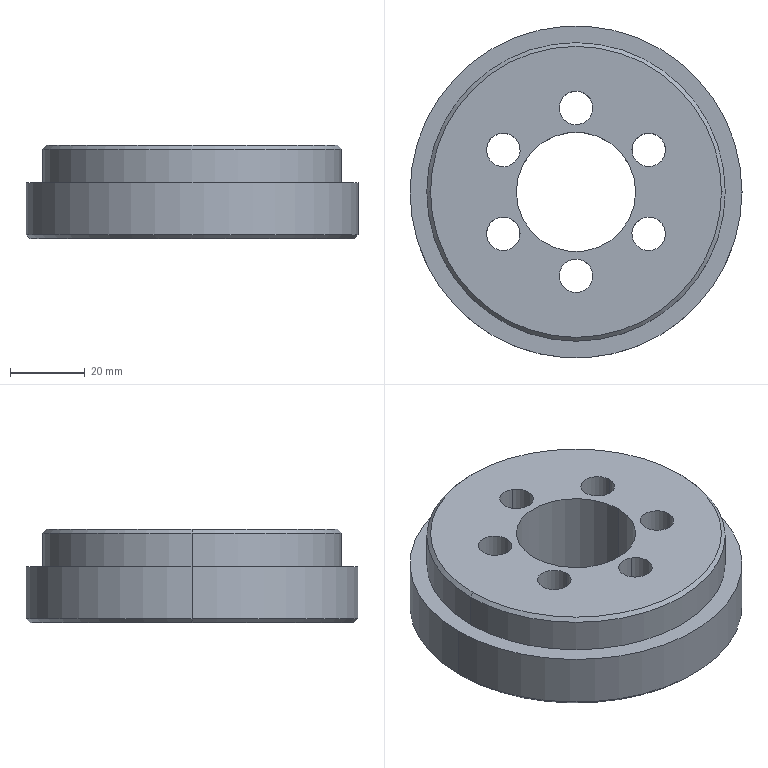Part | SolidWorks | features BaseBody 1 | 1 solid | 25 faces | box 89 x 89 x 25 mm | volume 113670 mm3 | cylinder 18 | cone 4 | plane 3 | commonest cylinder face diameters 9 x12 32 x2 80 x2 89 x2
STEP:
#1=CARTESIAN_POINT('',(-2.25,18.603,25.));
#2=VERTEX_POINT('',#1);
#3=CARTESIAN_POINT('',(2.25,26.397,25.));
#4=VERTEX_POINT('',#3);
#5=CARTESIAN_POINT('',(0.,22.5,25.));
#6=DIRECTION('',(0.,0.,1.));
#7=DIRECTION('',(0.5,0.866,0.));
#8=AXIS2_PLACEMENT_3D('',#5,#6,#7);
#9=CIRCLE('',#8,4.5);
#10=EDGE_CURVE('',#2,#4,#9,.T.);
#11=ORIENTED_EDGE('',*,*,#10,.T.);
#12=CARTESIAN_POINT('',(2.25,26.397,0.));
#13=VERTEX_POINT('',#12);
#14=CARTESIAN_POINT('',(2.25,26.397,0.));
#15=DIRECTION('',(0.,0.,-1.));
#16=VECTOR('',#15,1000.);
#17=LINE('',#14,#16);
#18=EDGE_CURVE('',#4,#13,#17,.T.);
#19=ORIENTED_EDGE('',*,*,#18,.T.);
#20=CARTESIAN_POINT('',(-2.25,18.603,0.));
#21=VERTEX_POINT('',#20);
#22=CARTESIAN_POINT('',(0.,22.5,0.));
#23=DIRECTION('',(0.,0.,-1.));
#24=DIRECTION('',(-0.5,-0.866,0.));
#25=AXIS2_PLACEMENT_3D('',#22,#23,#24);
#26=CIRCLE('',#25,4.5);
#27=EDGE_CURVE('',#13,#21,#26,.T.);
#28=ORIENTED_EDGE('',*,*,#27,.T.);
#29=CARTESIAN_POINT('',(-2.25,18.603,0.));
#30=DIRECTION('',(0.,0.,-1.));
#31=VECTOR('',#30,1000.);
#32=LINE('',#29,#31);
#33=EDGE_CURVE('',#2,#21,#32,.T.);
#34=ORIENTED_EDGE('',*,*,#33,.F.);
#35=EDGE_LOOP('',(#11,#19,#28,#34));
#36=FACE_OUTER_BOUND('',#35,.T.);
#37=CARTESIAN_POINT('',(0.,22.5,0.));
#38=DIRECTION('',(0.,0.,-1.));
#39=DIRECTION('',(-0.5,-0.866,0.));
#40=AXIS2_PLACEMENT_3D('',#37,#38,#39);
#41=CYLINDRICAL_SURFACE('',#40,4.5);
#42=ADVANCED_FACE('',(#36),#41,.F.);
#43=CARTESIAN_POINT('',(-17.236,7.353,25.));
#44=VERTEX_POINT('',#43);
#45=CARTESIAN_POINT('',(-21.736,15.147,25.));
#46=VERTEX_POINT('',#45);
#47=CARTESIAN_POINT('',(-19.486,11.25,25.));
#48=DIRECTION('',(0.,0.,1.));
#49=DIRECTION('',(-0.5,0.866,0.));
#50=AXIS2_PLACEMENT_3D('',#47,#48,#49);
#51=CIRCLE('',#50,4.5);
#52=EDGE_CURVE('',#44,#46,#51,.T.);
#53=ORIENTED_EDGE('',*,*,#52,.T.);
#54=CARTESIAN_POINT('',(-21.736,15.147,0.));
#55=VERTEX_POINT('',#54);
#56=CARTESIAN_POINT('',(-21.736,15.147,0.));
#57=DIRECTION('',(0.,0.,-1.));
#58=VECTOR('',#57,1000.);
#59=LINE('',#56,#58);
#60=EDGE_CURVE('',#46,#55,#59,.T.);
#61=ORIENTED_EDGE('',*,*,#60,.T.);
#62=CARTESIAN_POINT('',(-17.236,7.353,0.));
#63=VERTEX_POINT('',#62);
#64=CARTESIAN_POINT('',(-19.486,11.25,0.));
#65=DIRECTION('',(0.,0.,-1.));
#66=DIRECTION('',(0.5,-0.866,0.));
#67=AXIS2_PLACEMENT_3D('',#64,#65,#66);
#68=CIRCLE('',#67,4.5);
#69=EDGE_CURVE('',#55,#63,#68,.T.);
#70=ORIENTED_EDGE('',*,*,#69,.T.);
#71=CARTESIAN_POINT('',(-17.236,7.353,0.));
#72=DIRECTION('',(0.,0.,-1.));
#73=VECTOR('',#72,1000.);
#74=LINE('',#71,#73);
#75=EDGE_CURVE('',#44,#63,#74,.T.);
#76=ORIENTED_EDGE('',*,*,#75,.F.);
#77=EDGE_LOOP('',(#53,#61,#70,#76));
#78=FACE_OUTER_BOUND('',#77,.T.);
#79=CARTESIAN_POINT('',(-19.486,11.25,0.));
#80=DIRECTION('',(0.,0.,-1.));
#81=DIRECTION('',(0.5,-0.866,0.));
#82=AXIS2_PLACEMENT_3D('',#79,#80,#81);
#83=CYLINDRICAL_SURFACE('',#82,4.5);
#84=ADVANCED_FACE('',(#78),#83,.F.);
#85=CARTESIAN_POINT('',(-14.986,-11.25,25.));
#86=VERTEX_POINT('',#85);
#87=CARTESIAN_POINT('',(-23.986,-11.25,25.));
#88=VERTEX_POINT('',#87);
#89=CARTESIAN_POINT('',(-19.486,-11.25,25.));
#90=DIRECTION('',(0.,0.,1.));
#91=DIRECTION('',(-1.,0.,0.));
#92=AXIS2_PLACEMENT_3D('',#89,#90,#91);
#93=CIRCLE('',#92,4.5);
#94=EDGE_CURVE('',#86,#88,#93,.T.);
#95=ORIENTED_EDGE('',*,*,#94,.T.);
#96=CARTESIAN_POINT('',(-23.986,-11.25,0.));
#97=VERTEX_POINT('',#96);
#98=CARTESIAN_POINT('',(-23.986,-11.25,0.));
#99=DIRECTION('',(0.,0.,-1.));
#100=VECTOR('',#99,1000.);
#101=LINE('',#98,#100);
#102=EDGE_CURVE('',#88,#97,#101,.T.);
#103=ORIENTED_EDGE('',*,*,#102,.T.);
#104=CARTESIAN_POINT('',(-14.986,-11.25,0.));
#105=VERTEX_POINT('',#104);
#106=CARTESIAN_POINT('',(-19.486,-11.25,0.));
#107=DIRECTION('',(0.,0.,-1.));
#108=DIRECTION('',(1.,0.,0.));
#109=AXIS2_PLACEMENT_3D('',#106,#107,#108);
#110=CIRCLE('',#109,4.5);
#111=EDGE_CURVE('',#97,#105,#110,.T.);
#112=ORIENTED_EDGE('',*,*,#111,.T.);
#113=CARTESIAN_POINT('',(-14.986,-11.25,0.));
#114=DIRECTION('',(0.,0.,-1.));
#115=VECTOR('',#114,1000.);
#116=LINE('',#113,#115);
#117=EDGE_CURVE('',#86,#105,#116,.T.);
#118=ORIENTED_EDGE('',*,*,#117,.F.);
#119=EDGE_LOOP('',(#95,#103,#112,#118));
#120=FACE_OUTER_BOUND('',#119,.T.);
#121=CARTESIAN_POINT('',(-19.486,-11.25,0.));
#122=DIRECTION('',(0.,0.,-1.));
#123=DIRECTION('',(1.,0.,0.));
#124=AXIS2_PLACEMENT_3D('',#121,#122,#123);
#125=CYLINDRICAL_SURFACE('',#124,4.5);
#126=ADVANCED_FACE('',(#120),#125,.F.);
#127=CARTESIAN_POINT('',(2.25,-18.603,25.));
#128=VERTEX_POINT('',#127);
#129=CARTESIAN_POINT('',(-2.25,-26.397,25.));
#130=VERTEX_POINT('',#129);
#131=CARTESIAN_POINT('',(0.,-22.5,25.));
#132=DIRECTION('',(0.,0.,1.));
#133=DIRECTION('',(-0.5,-0.866,0.));
#134=AXIS2_PLACEMENT_3D('',#131,#132,#133);
#135=CIRCLE('',#134,4.5);
#136=EDGE_CURVE('',#128,#130,#135,.T.);
#137=ORIENTED_EDGE('',*,*,#136,.T.);
#138=CARTESIAN_POINT('',(-2.25,-26.397,0.));
#139=VERTEX_POINT('',#138);
#140=CARTESIAN_POINT('',(-2.25,-26.397,0.));
#141=DIRECTION('',(0.,0.,-1.));
#142=VECTOR('',#141,1000.);
#143=LINE('',#140,#142);
#144=EDGE_CURVE('',#130,#139,#143,.T.);
#145=ORIENTED_EDGE('',*,*,#144,.T.);
#146=CARTESIAN_POINT('',(2.25,-18.603,0.));
#147=VERTEX_POINT('',#146);
#148=CARTESIAN_POINT('',(0.,-22.5,0.));
#149=DIRECTION('',(0.,0.,-1.));
#150=DIRECTION('',(0.5,0.866,0.));
#151=AXIS2_PLACEMENT_3D('',#148,#149,#150);
#152=CIRCLE('',#151,4.5);
#153=EDGE_CURVE('',#139,#147,#152,.T.);
#154=ORIENTED_EDGE('',*,*,#153,.T.);
#155=CARTESIAN_POINT('',(2.25,-18.603,0.));
#156=DIRECTION('',(0.,0.,-1.));
#157=VECTOR('',#156,1000.);
#158=LINE('',#155,#157);
#159=EDGE_CURVE('',#128,#147,#158,.T.);
#160=ORIENTED_EDGE('',*,*,#159,.F.);
#161=EDGE_LOOP('',(#137,#145,#154,#160));
#162=FACE_OUTER_BOUND('',#161,.T.);
#163=CARTESIAN_POINT('',(0.,-22.5,0.));
#164=DIRECTION('',(0.,0.,-1.));
#165=DIRECTION('',(0.5,0.866,0.));
#166=AXIS2_PLACEMENT_3D('',#163,#164,#165);
#167=CYLINDRICAL_SURFACE('',#166,4.5);
#168=ADVANCED_FACE('',(#162),#167,.F.);
#169=CARTESIAN_POINT('',(17.236,-7.353,25.));
#170=VERTEX_POINT('',#169);
#171=CARTESIAN_POINT('',(21.736,-15.147,25.));
#172=VERTEX_POINT('',#171);
#173=CARTESIAN_POINT('',(19.486,-11.25,25.));
#174=DIRECTION('',(0.,0.,1.));
#175=DIRECTION('',(0.5,-0.866,0.));
#176=AXIS2_PLACEMENT_3D('',#173,#174,#175);
#177=CIRCLE('',#176,4.5);
#178=EDGE_CURVE('',#170,#172,#177,.T.);
#179=ORIENTED_EDGE('',*,*,#178,.T.);
#180=CARTESIAN_POINT('',(21.736,-15.147,0.));
#181=VERTEX_POINT('',#180);
#182=CARTESIAN_POINT('',(21.736,-15.147,0.));
#183=DIRECTION('',(0.,0.,-1.));
#184=VECTOR('',#183,1000.);
#185=LINE('',#182,#184);
#186=EDGE_CURVE('',#172,#181,#185,.T.);
#187=ORIENTED_EDGE('',*,*,#186,.T.);
#188=CARTESIAN_POINT('',(17.236,-7.353,0.));
#189=VERTEX_POINT('',#188);
#190=CARTESIAN_POINT('',(19.486,-11.25,0.));
#191=DIRECTION('',(0.,0.,-1.));
#192=DIRECTION('',(-0.5,0.866,0.));
#193=AXIS2_PLACEMENT_3D('',#190,#191,#192);
#194=CIRCLE('',#193,4.5);
#195=EDGE_CURVE('',#181,#189,#194,.T.);
#196=ORIENTED_EDGE('',*,*,#195,.T.);
#197=CARTESIAN_POINT('',(17.236,-7.353,0.));
#198=DIRECTION('',(0.,0.,-1.));
#199=VECTOR('',#198,1000.);
#200=LINE('',#197,#199);
#201=EDGE_CURVE('',#170,#189,#200,.T.);
#202=ORIENTED_EDGE('',*,*,#201,.F.);
#203=EDGE_LOOP('',(#179,#187,#196,#202));
#204=FACE_OUTER_BOUND('',#203,.T.);
#205=CARTESIAN_POINT('',(19.486,-11.25,0.));
#206=DIRECTION('',(0.,0.,-1.));
#207=DIRECTION('',(-0.5,0.866,0.));
#208=AXIS2_PLACEMENT_3D('',#205,#206,#207);
#209=CYLINDRICAL_SURFACE('',#208,4.5);
#210=ADVANCED_FACE('',(#204),#209,.F.);
#211=CARTESIAN_POINT('',(14.986,11.25,25.));
#212=VERTEX_POINT('',#211);
#213=CARTESIAN_POINT('',(23.986,11.25,25.));
#214=VERTEX_POINT('',#213);
#215=CARTESIAN_POINT('',(19.486,11.25,25.));
#216=DIRECTION('',(0.,0.,1.));
#217=DIRECTION('',(1.,0.,0.));
#218=AXIS2_PLACEMENT_3D('',#215,#216,#217);
#219=CIRCLE('',#218,4.5);
#220=EDGE_CURVE('',#212,#214,#219,.T.);
#221=ORIENTED_EDGE('',*,*,#220,.T.);
#222=CARTESIAN_POINT('',(23.986,11.25,0.));
#223=VERTEX_POINT('',#222);
#224=CARTESIAN_POINT('',(23.986,11.25,0.));
#225=DIRECTION('',(0.,0.,-1.));
#226=VECTOR('',#225,1000.);
#227=LINE('',#224,#226);
#228=EDGE_CURVE('',#214,#223,#227,.T.);
#229=ORIENTED_EDGE('',*,*,#228,.T.);
#230=CARTESIAN_POINT('',(14.986,11.25,0.));
#231=VERTEX_POINT('',#230);
#232=CARTESIAN_POINT('',(19.486,11.25,0.));
#233=DIRECTION('',(0.,0.,-1.));
#234=DIRECTION('',(-1.,0.,0.));
#235=AXIS2_PLACEMENT_3D('',#232,#233,#234);
#236=CIRCLE('',#235,4.5);
#237=EDGE_CURVE('',#223,#231,#236,.T.);
#238=ORIENTED_EDGE('',*,*,#237,.T.);
#239=CARTESIAN_POINT('',(14.986,11.25,0.));
#240=DIRECTION('',(0.,0.,-1.));
#241=VECTOR('',#240,1000.);
#242=LINE('',#239,#241);
#243=EDGE_CURVE('',#212,#231,#242,.T.);
#244=ORIENTED_EDGE('',*,*,#243,.F.);
#245=EDGE_LOOP('',(#221,#229,#238,#244));
#246=FACE_OUTER_BOUND('',#245,.T.);
#247=CARTESIAN_POINT('',(19.486,11.25,0.));
#248=DIRECTION('',(0.,0.,-1.));
#249=DIRECTION('',(-1.,0.,0.));
#250=AXIS2_PLACEMENT_3D('',#247,#248,#249);
#251=CYLINDRICAL_SURFACE('',#250,4.5);
#252=ADVANCED_FACE('',(#246),#251,.F.);
#253=CARTESIAN_POINT('',(-16.,0.,0.));
#254=VERTEX_POINT('',#253);
#255=CARTESIAN_POINT('',(16.,0.,0.));
#256=VERTEX_POINT('',#255);
#257=CARTESIAN_POINT('',(0.,0.,0.));
#258=DIRECTION('',(0.,0.,1.));
#259=DIRECTION('',(1.,0.,0.));
#260=AXIS2_PLACEMENT_3D('',#257,#258,#259);
#261=CIRCLE('',#260,16.);
#262=EDGE_CURVE('',#254,#256,#261,.T.);
#263=ORIENTED_EDGE('',*,*,#262,.F.);
#264=CARTESIAN_POINT('',(-16.,0.,25.));
#265=VERTEX_POINT('',#264);
#266=CARTESIAN_POINT('',(-16.,0.,0.));
#267=DIRECTION('',(0.,0.,1.));
#268=VECTOR('',#267,1000.);
#269=LINE('',#266,#268);
#270=EDGE_CURVE('',#254,#265,#269,.T.);
#271=ORIENTED_EDGE('',*,*,#270,.T.);
#272=CARTESIAN_POINT('',(16.,0.,25.));
#273=VERTEX_POINT('',#272);
#274=CARTESIAN_POINT('',(0.,0.,25.));
#275=DIRECTION('',(0.,0.,1.));
#276=DIRECTION('',(1.,0.,0.));
#277=AXIS2_PLACEMENT_3D('',#274,#275,#276);
#278=CIRCLE('',#277,16.);
#279=EDGE_CURVE('',#265,#273,#278,.T.);
#280=ORIENTED_EDGE('',*,*,#279,.T.);
#281=CARTESIAN_POINT('',(16.,0.,0.));
#282=DIRECTION('',(0.,0.,1.));
#283=VECTOR('',#282,1000.);
#284=LINE('',#281,#283);
#285=EDGE_CURVE('',#256,#273,#284,.T.);
#286=ORIENTED_EDGE('',*,*,#285,.F.);
#287=EDGE_LOOP('',(#263,#271,#280,#286));
#288=FACE_OUTER_BOUND('',#287,.T.);
#289=CARTESIAN_POINT('',(0.,0.,0.));
#290=DIRECTION('',(0.,0.,1.));
#291=DIRECTION('',(1.,0.,0.));
#292=AXIS2_PLACEMENT_3D('',#289,#290,#291);
#293=CYLINDRICAL_SURFACE('',#292,16.);
#294=ADVANCED_FACE('',(#288),#293,.F.);
#295=CARTESIAN_POINT('',(39.,0.,25.));
#296=VERTEX_POINT('',#295);
#297=CARTESIAN_POINT('',(-39.,0.,25.));
#298=VERTEX_POINT('',#297);
#299=CARTESIAN_POINT('',(0.,0.,25.));
#300=DIRECTION('',(0.,0.,1.));
#301=DIRECTION('',(1.,0.,0.));
#302=AXIS2_PLACEMENT_3D('',#299,#300,#301);
#303=CIRCLE('',#302,39.);
#304=EDGE_CURVE('',#296,#298,#303,.T.);
#305=ORIENTED_EDGE('',*,*,#304,.F.);
#306=CARTESIAN_POINT('',(40.,0.,24.));
#307=VERTEX_POINT('',#306);
#308=CARTESIAN_POINT('',(39.,0.,25.));
#309=DIRECTION('',(0.7071,0.,-0.7071));
#310=VECTOR('',#309,1000.);
#311=LINE('',#308,#310);
#312=EDGE_CURVE('',#296,#307,#311,.T.);
#313=ORIENTED_EDGE('',*,*,#312,.T.);
#314=CARTESIAN_POINT('',(-40.,0.,24.));
#315=VERTEX_POINT('',#314);
#316=CARTESIAN_POINT('',(0.,0.,24.));
#317=DIRECTION('',(0.,0.,-1.));
#318=DIRECTION('',(1.,0.,0.));
#319=AXIS2_PLACEMENT_3D('',#316,#317,#318);
#320=CIRCLE('',#319,40.);
#321=EDGE_CURVE('',#315,#307,#320,.T.);
#322=ORIENTED_EDGE('',*,*,#321,.F.);
#323=CARTESIAN_POINT('',(-39.,0.,25.));
#324=DIRECTION('',(-0.7071,0.,-0.7071));
#325=VECTOR('',#324,1000.);
#326=LINE('',#323,#325);
#327=EDGE_CURVE('',#298,#315,#326,.T.);
#328=ORIENTED_EDGE('',*,*,#327,.F.);
#329=EDGE_LOOP('',(#305,#313,#322,#328));
#330=FACE_OUTER_BOUND('',#329,.T.);
#331=CARTESIAN_POINT('',(0.,0.,25.));
#332=DIRECTION('',(0.,0.,-1.));
#333=DIRECTION('',(-1.,0.,0.));
#334=AXIS2_PLACEMENT_3D('',#331,#332,#333);
#335=CONICAL_SURFACE('',#334,39.,0.7854);
#336=ADVANCED_FACE('',(#330),#335,.T.);
#337=CARTESIAN_POINT('',(-43.5,0.,0.));
#338=VERTEX_POINT('',#337);
#339=CARTESIAN_POINT('',(43.5,0.,0.));
#340=VERTEX_POINT('',#339);
#341=CARTESIAN_POINT('',(0.,0.,0.));
#342=DIRECTION('',(0.,0.,-1.));
#343=DIRECTION('',(1.,0.,0.));
#344=AXIS2_PLACEMENT_3D('',#341,#342,#343);
#345=CIRCLE('',#344,43.5);
#346=EDGE_CURVE('',#338,#340,#345,.T.);
#347=ORIENTED_EDGE('',*,*,#346,.F.);
#348=CARTESIAN_POINT('',(-44.5,0.,1.));
#349=VERTEX_POINT('',#348);
#350=CARTESIAN_POINT('',(-44.5,0.,1.));
#351=DIRECTION('',(-0.7071,0.,0.7071));
#352=VECTOR('',#351,1000.);
#353=LINE('',#350,#352);
#354=EDGE_CURVE('',#338,#349,#353,.T.);
#355=ORIENTED_EDGE('',*,*,#354,.T.);
#356=CARTESIAN_POINT('',(44.5,0.,1.));
#357=VERTEX_POINT('',#356);
#358=CARTESIAN_POINT('',(0.,0.,1.));
#359=DIRECTION('',(0.,0.,1.));
#360=DIRECTION('',(1.,0.,0.));
#361=AXIS2_PLACEMENT_3D('',#358,#359,#360);
#362=CIRCLE('',#361,44.5);
#363=EDGE_CURVE('',#357,#349,#362,.T.);
#364=ORIENTED_EDGE('',*,*,#363,.F.);
#365=CARTESIAN_POINT('',(44.5,0.,1.));
#366=DIRECTION('',(0.7071,0.,0.7071));
#367=VECTOR('',#366,1000.);
#368=LINE('',#365,#367);
#369=EDGE_CURVE('',#340,#357,#368,.T.);
#370=ORIENTED_EDGE('',*,*,#369,.F.);
#371=EDGE_LOOP('',(#347,#355,#364,#370));
#372=FACE_OUTER_BOUND('',#371,.T.);
#373=CARTESIAN_POINT('',(0.,0.,1.));
#374=DIRECTION('',(0.,0.,1.));
#375=DIRECTION('',(1.,0.,0.));
#376=AXIS2_PLACEMENT_3D('',#373,#374,#375);
#377=CONICAL_SURFACE('',#376,44.5,0.7854);
#378=ADVANCED_FACE('',(#372),#377,.T.);
#379=ORIENTED_EDGE('',*,*,#321,.T.);
#380=CARTESIAN_POINT('',(40.,0.,15.));
#381=VERTEX_POINT('',#380);
#382=CARTESIAN_POINT('',(40.,0.,25.));
#383=DIRECTION('',(0.,0.,-1.));
#384=VECTOR('',#383,1000.);
#385=LINE('',#382,#384);
#386=EDGE_CURVE('',#307,#381,#385,.T.);
#387=ORIENTED_EDGE('',*,*,#386,.T.);
#388=CARTESIAN_POINT('',(-40.,0.,15.));
#389=VERTEX_POINT('',#388);
#390=CARTESIAN_POINT('',(0.,0.,15.));
#391=DIRECTION('',(0.,0.,1.));
#392=DIRECTION('',(1.,0.,0.));
#393=AXIS2_PLACEMENT_3D('',#390,#391,#392);
#394=CIRCLE('',#393,40.);
#395=EDGE_CURVE('',#381,#389,#394,.T.);
#396=ORIENTED_EDGE('',*,*,#395,.T.);
#397=CARTESIAN_POINT('',(-40.,0.,25.));
#398=DIRECTION('',(0.,0.,-1.));
#399=VECTOR('',#398,1000.);
#400=LINE('',#397,#399);
#401=EDGE_CURVE('',#315,#389,#400,.T.);
#402=ORIENTED_EDGE('',*,*,#401,.F.);
#403=EDGE_LOOP('',(#379,#387,#396,#402));
#404=FACE_OUTER_BOUND('',#403,.T.);
#405=CARTESIAN_POINT('',(0.,0.,25.));
#406=DIRECTION('',(0.,0.,-1.));
#407=DIRECTION('',(-1.,0.,0.));
#408=AXIS2_PLACEMENT_3D('',#405,#406,#407);
#409=CYLINDRICAL_SURFACE('',#408,40.);
#410=ADVANCED_FACE('',(#404),#409,.T.);
#411=CARTESIAN_POINT('',(44.5,0.,15.));
#412=VERTEX_POINT('',#411);
#413=CARTESIAN_POINT('',(-44.5,0.,15.));
#414=VERTEX_POINT('',#413);
#415=CARTESIAN_POINT('',(0.,0.,15.));
#416=DIRECTION('',(0.,0.,1.));
#417=DIRECTION('',(1.,0.,0.));
#418=AXIS2_PLACEMENT_3D('',#415,#416,#417);
#419=CIRCLE('',#418,44.5);
#420=EDGE_CURVE('',#412,#414,#419,.T.);
#421=ORIENTED_EDGE('',*,*,#420,.F.);
#422=CARTESIAN_POINT('',(44.5,0.,15.));
#423=DIRECTION('',(0.,0.,-1.));
#424=VECTOR('',#423,1000.);
#425=LINE('',#422,#424);
#426=EDGE_CURVE('',#412,#357,#425,.T.);
#427=ORIENTED_EDGE('',*,*,#426,.T.);
#428=ORIENTED_EDGE('',*,*,#363,.T.);
#429=CARTESIAN_POINT('',(-44.5,0.,15.));
#430=DIRECTION('',(0.,0.,-1.));
#431=VECTOR('',#430,1000.);
#432=LINE('',#429,#431);
#433=EDGE_CURVE('',#414,#349,#432,.T.);
#434=ORIENTED_EDGE('',*,*,#433,.F.);
#435=EDGE_LOOP('',(#421,#427,#428,#434));
#436=FACE_OUTER_BOUND('',#435,.T.);
#437=CARTESIAN_POINT('',(0.,0.,15.));
#438=DIRECTION('',(0.,0.,-1.));
#439=DIRECTION('',(-1.,0.,0.));
#440=AXIS2_PLACEMENT_3D('',#437,#438,#439);
#441=CYLINDRICAL_SURFACE('',#440,44.5);
#442=ADVANCED_FACE('',(#436),#441,.T.);
#443=ORIENTED_EDGE('',*,*,#426,.F.);
#444=CARTESIAN_POINT('',(0.,0.,15.));
#445=DIRECTION('',(0.,0.,1.));
#446=DIRECTION('',(1.,0.,0.));
#447=AXIS2_PLACEMENT_3D('',#444,#445,#446);
#448=CIRCLE('',#447,44.5);
#449=EDGE_CURVE('',#414,#412,#448,.T.);
#450=ORIENTED_EDGE('',*,*,#449,.F.);
#451=ORIENTED_EDGE('',*,*,#433,.T.);
#452=CARTESIAN_POINT('',(0.,0.,1.));
#453=DIRECTION('',(0.,0.,1.));
#454=DIRECTION('',(1.,0.,0.));
#455=AXIS2_PLACEMENT_3D('',#452,#453,#454);
#456=CIRCLE('',#455,44.5);
#457=EDGE_CURVE('',#349,#357,#456,.T.);
#458=ORIENTED_EDGE('',*,*,#457,.T.);
#459=EDGE_LOOP('',(#443,#450,#451,#458));
#460=FACE_OUTER_BOUND('',#459,.T.);
#461=CARTESIAN_POINT('',(0.,0.,15.));
#462=DIRECTION('',(0.,0.,-1.));
#463=DIRECTION('',(-1.,0.,0.));
#464=AXIS2_PLACEMENT_3D('',#461,#462,#463);
#465=CYLINDRICAL_SURFACE('',#464,44.5);
#466=ADVANCED_FACE('',(#460),#465,.T.);
#467=CARTESIAN_POINT('',(0.,0.,15.));
#468=DIRECTION('',(0.,0.,1.));
#469=DIRECTION('',(1.,0.,0.));
#470=AXIS2_PLACEMENT_3D('',#467,#468,#469);
#471=CIRCLE('',#470,40.);
#472=EDGE_CURVE('',#389,#381,#471,.T.);
#473=ORIENTED_EDGE('',*,*,#472,.F.);
#474=ORIENTED_EDGE('',*,*,#395,.F.);
#475=EDGE_LOOP('',(#473,#474));
#476=FACE_BOUND('',#475,.T.);
#477=ORIENTED_EDGE('',*,*,#449,.T.);
#478=ORIENTED_EDGE('',*,*,#420,.T.);
#479=EDGE_LOOP('',(#477,#478));
#480=FACE_OUTER_BOUND('',#479,.T.);
#481=CARTESIAN_POINT('',(0.,0.,15.));
#482=DIRECTION('',(0.,0.,1.));
#483=DIRECTION('',(1.,0.,0.));
#484=AXIS2_PLACEMENT_3D('',#481,#482,#483);
#485=PLANE('',#484);
#486=ADVANCED_FACE('',(#476,#480),#485,.T.);
#487=CARTESIAN_POINT('',(0.,22.5,0.));
#488=DIRECTION('',(0.,0.,-1.));
#489=DIRECTION('',(-0.5,-0.866,0.));
#490=AXIS2_PLACEMENT_3D('',#487,#488,#489);
#491=CIRCLE('',#490,4.5);
#492=EDGE_CURVE('',#21,#13,#491,.T.);
#493=ORIENTED_EDGE('',*,*,#492,.F.);
#494=ORIENTED_EDGE('',*,*,#27,.F.);
#495=EDGE_LOOP('',(#493,#494));
#496=FACE_BOUND('',#495,.T.);
#497=CARTESIAN_POINT('',(-19.486,11.25,0.));
#498=DIRECTION('',(0.,0.,-1.));
#499=DIRECTION('',(0.5,-0.866,0.));
#500=AXIS2_PLACEMENT_3D('',#497,#498,#499);
#501=CIRCLE('',#500,4.5);
#502=EDGE_CURVE('',#63,#55,#501,.T.);
#503=ORIENTED_EDGE('',*,*,#502,.F.);
#504=ORIENTED_EDGE('',*,*,#69,.F.);
#505=EDGE_LOOP('',(#503,#504));
#506=FACE_BOUND('',#505,.T.);
#507=CARTESIAN_POINT('',(-19.486,-11.25,0.));
#508=DIRECTION('',(0.,0.,-1.));
#509=DIRECTION('',(1.,0.,0.));
#510=AXIS2_PLACEMENT_3D('',#507,#508,#509);
#511=CIRCLE('',#510,4.5);
#512=EDGE_CURVE('',#105,#97,#511,.T.);
#513=ORIENTED_EDGE('',*,*,#512,.F.);
#514=ORIENTED_EDGE('',*,*,#111,.F.);
#515=EDGE_LOOP('',(#513,#514));
#516=FACE_BOUND('',#515,.T.);
#517=CARTESIAN_POINT('',(0.,-22.5,0.));
#518=DIRECTION('',(0.,0.,-1.));
#519=DIRECTION('',(0.5,0.866,0.));
#520=AXIS2_PLACEMENT_3D('',#517,#518,#519);
#521=CIRCLE('',#520,4.5);
#522=EDGE_CURVE('',#147,#139,#521,.T.);
#523=ORIENTED_EDGE('',*,*,#522,.F.);
#524=ORIENTED_EDGE('',*,*,#153,.F.);
#525=EDGE_LOOP('',(#523,#524));
#526=FACE_BOUND('',#525,.T.);
#527=CARTESIAN_POINT('',(19.486,-11.25,0.));
#528=DIRECTION('',(0.,0.,-1.));
#529=DIRECTION('',(-0.5,0.866,0.));
#530=AXIS2_PLACEMENT_3D('',#527,#528,#529);
#531=CIRCLE('',#530,4.5);
#532=EDGE_CURVE('',#189,#181,#531,.T.);
#533=ORIENTED_EDGE('',*,*,#532,.F.);
#534=ORIENTED_EDGE('',*,*,#195,.F.);
#535=EDGE_LOOP('',(#533,#534));
#536=FACE_BOUND('',#535,.T.);
#537=CARTESIAN_POINT('',(19.486,11.25,0.));
#538=DIRECTION('',(0.,0.,-1.));
#539=DIRECTION('',(-1.,0.,0.));
#540=AXIS2_PLACEMENT_3D('',#537,#538,#539);
#541=CIRCLE('',#540,4.5);
#542=EDGE_CURVE('',#231,#223,#541,.T.);
#543=ORIENTED_EDGE('',*,*,#542,.F.);
#544=ORIENTED_EDGE('',*,*,#237,.F.);
#545=EDGE_LOOP('',(#543,#544));
#546=FACE_BOUND('',#545,.T.);
#547=CARTESIAN_POINT('',(0.,0.,0.));
#548=DIRECTION('',(0.,0.,1.));
#549=DIRECTION('',(1.,0.,0.));
#550=AXIS2_PLACEMENT_3D('',#547,#548,#549);
#551=CIRCLE('',#550,16.);
#552=EDGE_CURVE('',#256,#254,#551,.T.);
#553=ORIENTED_EDGE('',*,*,#552,.T.);
#554=ORIENTED_EDGE('',*,*,#262,.T.);
#555=EDGE_LOOP('',(#553,#554));
#556=FACE_BOUND('',#555,.T.);
#557=CARTESIAN_POINT('',(0.,0.,0.));
#558=DIRECTION('',(0.,0.,-1.));
#559=DIRECTION('',(1.,0.,0.));
#560=AXIS2_PLACEMENT_3D('',#557,#558,#559);
#561=CIRCLE('',#560,43.5);
#562=EDGE_CURVE('',#340,#338,#561,.T.);
#563=ORIENTED_EDGE('',*,*,#562,.T.);
#564=ORIENTED_EDGE('',*,*,#346,.T.);
#565=EDGE_LOOP('',(#563,#564));
#566=FACE_OUTER_BOUND('',#565,.T.);
#567=CARTESIAN_POINT('',(0.,0.,0.));
#568=DIRECTION('',(0.,0.,1.));
#569=DIRECTION('',(1.,0.,0.));
#570=AXIS2_PLACEMENT_3D('',#567,#568,#569);
#571=PLANE('',#570);
#572=ADVANCED_FACE('',(#496,#506,#516,#526,#536,#546,#556,#566),#571,.F.);
#573=ORIENTED_EDGE('',*,*,#386,.F.);
#574=CARTESIAN_POINT('',(0.,0.,24.));
#575=DIRECTION('',(0.,0.,-1.));
#576=DIRECTION('',(1.,0.,0.));
#577=AXIS2_PLACEMENT_3D('',#574,#575,#576);
#578=CIRCLE('',#577,40.);
#579=EDGE_CURVE('',#307,#315,#578,.T.);
#580=ORIENTED_EDGE('',*,*,#579,.T.);
#581=ORIENTED_EDGE('',*,*,#401,.T.);
#582=ORIENTED_EDGE('',*,*,#472,.T.);
#583=EDGE_LOOP('',(#573,#580,#581,#582));
#584=FACE_OUTER_BOUND('',#583,.T.);
#585=CARTESIAN_POINT('',(0.,0.,25.));
#586=DIRECTION('',(0.,0.,-1.));
#587=DIRECTION('',(-1.,0.,0.));
#588=AXIS2_PLACEMENT_3D('',#585,#586,#587);
#589=CYLINDRICAL_SURFACE('',#588,40.);
#590=ADVANCED_FACE('',(#584),#589,.T.);
#591=ORIENTED_EDGE('',*,*,#10,.F.);
#592=CARTESIAN_POINT('',(0.,22.5,25.));
#593=DIRECTION('',(0.,0.,1.));
#594=DIRECTION('',(0.5,0.866,0.));
#595=AXIS2_PLACEMENT_3D('',#592,#593,#594);
#596=CIRCLE('',#595,4.5);
#597=EDGE_CURVE('',#4,#2,#596,.T.);
#598=ORIENTED_EDGE('',*,*,#597,.F.);
#599=EDGE_LOOP('',(#591,#598));
#600=FACE_BOUND('',#599,.T.);
#601=ORIENTED_EDGE('',*,*,#52,.F.);
#602=CARTESIAN_POINT('',(-19.486,11.25,25.));
#603=DIRECTION('',(0.,0.,1.));
#604=DIRECTION('',(-0.5,0.866,0.));
#605=AXIS2_PLACEMENT_3D('',#602,#603,#604);
#606=CIRCLE('',#605,4.5);
#607=EDGE_CURVE('',#46,#44,#606,.T.);
#608=ORIENTED_EDGE('',*,*,#607,.F.);
#609=EDGE_LOOP('',(#601,#608));
#610=FACE_BOUND('',#609,.T.);
#611=ORIENTED_EDGE('',*,*,#94,.F.);
#612=CARTESIAN_POINT('',(-19.486,-11.25,25.));
#613=DIRECTION('',(0.,0.,1.));
#614=DIRECTION('',(-1.,0.,0.));
#615=AXIS2_PLACEMENT_3D('',#612,#613,#614);
#616=CIRCLE('',#615,4.5);
#617=EDGE_CURVE('',#88,#86,#616,.T.);
#618=ORIENTED_EDGE('',*,*,#617,.F.);
#619=EDGE_LOOP('',(#611,#618));
#620=FACE_BOUND('',#619,.T.);
#621=ORIENTED_EDGE('',*,*,#136,.F.);
#622=CARTESIAN_POINT('',(0.,-22.5,25.));
#623=DIRECTION('',(0.,0.,1.));
#624=DIRECTION('',(-0.5,-0.866,0.));
#625=AXIS2_PLACEMENT_3D('',#622,#623,#624);
#626=CIRCLE('',#625,4.5);
#627=EDGE_CURVE('',#130,#128,#626,.T.);
#628=ORIENTED_EDGE('',*,*,#627,.F.);
#629=EDGE_LOOP('',(#621,#628));
#630=FACE_BOUND('',#629,.T.);
#631=ORIENTED_EDGE('',*,*,#178,.F.);
#632=CARTESIAN_POINT('',(19.486,-11.25,25.));
#633=DIRECTION('',(0.,0.,1.));
#634=DIRECTION('',(0.5,-0.866,0.));
#635=AXIS2_PLACEMENT_3D('',#632,#633,#634);
#636=CIRCLE('',#635,4.5);
#637=EDGE_CURVE('',#172,#170,#636,.T.);
#638=ORIENTED_EDGE('',*,*,#637,.F.);
#639=EDGE_LOOP('',(#631,#638));
#640=FACE_BOUND('',#639,.T.);
#641=ORIENTED_EDGE('',*,*,#220,.F.);
#642=CARTESIAN_POINT('',(19.486,11.25,25.));
#643=DIRECTION('',(0.,0.,1.));
#644=DIRECTION('',(1.,0.,0.));
#645=AXIS2_PLACEMENT_3D('',#642,#643,#644);
#646=CIRCLE('',#645,4.5);
#647=EDGE_CURVE('',#214,#212,#646,.T.);
#648=ORIENTED_EDGE('',*,*,#647,.F.);
#649=EDGE_LOOP('',(#641,#648));
#650=FACE_BOUND('',#649,.T.);
#651=CARTESIAN_POINT('',(0.,0.,25.));
#652=DIRECTION('',(0.,0.,1.));
#653=DIRECTION('',(1.,0.,0.));
#654=AXIS2_PLACEMENT_3D('',#651,#652,#653);
#655=CIRCLE('',#654,16.);
#656=EDGE_CURVE('',#273,#265,#655,.T.);
#657=ORIENTED_EDGE('',*,*,#656,.F.);
#658=ORIENTED_EDGE('',*,*,#279,.F.);
#659=EDGE_LOOP('',(#657,#658));
#660=FACE_BOUND('',#659,.T.);
#661=CARTESIAN_POINT('',(0.,0.,25.));
#662=DIRECTION('',(0.,0.,1.));
#663=DIRECTION('',(1.,0.,0.));
#664=AXIS2_PLACEMENT_3D('',#661,#662,#663);
#665=CIRCLE('',#664,39.);
#666=EDGE_CURVE('',#298,#296,#665,.T.);
#667=ORIENTED_EDGE('',*,*,#666,.T.);
#668=ORIENTED_EDGE('',*,*,#304,.T.);
#669=EDGE_LOOP('',(#667,#668));
#670=FACE_OUTER_BOUND('',#669,.T.);
#671=CARTESIAN_POINT('',(0.,0.,25.));
#672=DIRECTION('',(0.,0.,1.));
#673=DIRECTION('',(1.,0.,0.));
#674=AXIS2_PLACEMENT_3D('',#671,#672,#673);
#675=PLANE('',#674);
#676=ADVANCED_FACE('',(#600,#610,#620,#630,#640,#650,#660,#670),#675,.T.);
#677=ORIENTED_EDGE('',*,*,#354,.F.);
#678=ORIENTED_EDGE('',*,*,#562,.F.);
#679=ORIENTED_EDGE('',*,*,#369,.T.);
#680=ORIENTED_EDGE('',*,*,#457,.F.);
#681=EDGE_LOOP('',(#677,#678,#679,#680));
#682=FACE_OUTER_BOUND('',#681,.T.);
#683=CARTESIAN_POINT('',(0.,0.,1.));
#684=DIRECTION('',(0.,0.,1.));
#685=DIRECTION('',(1.,0.,0.));
#686=AXIS2_PLACEMENT_3D('',#683,#684,#685);
#687=CONICAL_SURFACE('',#686,44.5,0.7854);
#688=ADVANCED_FACE('',(#682),#687,.T.);
#689=ORIENTED_EDGE('',*,*,#312,.F.);
#690=ORIENTED_EDGE('',*,*,#666,.F.);
#691=ORIENTED_EDGE('',*,*,#327,.T.);
#692=ORIENTED_EDGE('',*,*,#579,.F.);
#693=EDGE_LOOP('',(#689,#690,#691,#692));
#694=FACE_OUTER_BOUND('',#693,.T.);
#695=CARTESIAN_POINT('',(0.,0.,25.));
#696=DIRECTION('',(0.,0.,-1.));
#697=DIRECTION('',(-1.,0.,0.));
#698=AXIS2_PLACEMENT_3D('',#695,#696,#697);
#699=CONICAL_SURFACE('',#698,39.,0.7854);
#700=ADVANCED_FACE('',(#694),#699,.T.);
#701=ORIENTED_EDGE('',*,*,#270,.F.);
#702=ORIENTED_EDGE('',*,*,#552,.F.);
#703=ORIENTED_EDGE('',*,*,#285,.T.);
#704=ORIENTED_EDGE('',*,*,#656,.T.);
#705=EDGE_LOOP('',(#701,#702,#703,#704));
#706=FACE_OUTER_BOUND('',#705,.T.);
#707=CARTESIAN_POINT('',(0.,0.,0.));
#708=DIRECTION('',(0.,0.,1.));
#709=DIRECTION('',(1.,0.,0.));
#710=AXIS2_PLACEMENT_3D('',#707,#708,#709);
#711=CYLINDRICAL_SURFACE('',#710,16.);
#712=ADVANCED_FACE('',(#706),#711,.F.);
#713=ORIENTED_EDGE('',*,*,#228,.F.);
#714=ORIENTED_EDGE('',*,*,#647,.T.);
#715=ORIENTED_EDGE('',*,*,#243,.T.);
#716=ORIENTED_EDGE('',*,*,#542,.T.);
#717=EDGE_LOOP('',(#713,#714,#715,#716));
#718=FACE_OUTER_BOUND('',#717,.T.);
#719=CARTESIAN_POINT('',(19.486,11.25,0.));
#720=DIRECTION('',(0.,0.,-1.));
#721=DIRECTION('',(-1.,0.,0.));
#722=AXIS2_PLACEMENT_3D('',#719,#720,#721);
#723=CYLINDRICAL_SURFACE('',#722,4.5);
#724=ADVANCED_FACE('',(#718),#723,.F.);
#725=ORIENTED_EDGE('',*,*,#186,.F.);
#726=ORIENTED_EDGE('',*,*,#637,.T.);
#727=ORIENTED_EDGE('',*,*,#201,.T.);
#728=ORIENTED_EDGE('',*,*,#532,.T.);
#729=EDGE_LOOP('',(#725,#726,#727,#728));
#730=FACE_OUTER_BOUND('',#729,.T.);
#731=CARTESIAN_POINT('',(19.486,-11.25,0.));
#732=DIRECTION('',(0.,0.,-1.));
#733=DIRECTION('',(-0.5,0.866,0.));
#734=AXIS2_PLACEMENT_3D('',#731,#732,#733);
#735=CYLINDRICAL_SURFACE('',#734,4.5);
#736=ADVANCED_FACE('',(#730),#735,.F.);
#737=ORIENTED_EDGE('',*,*,#144,.F.);
#738=ORIENTED_EDGE('',*,*,#627,.T.);
#739=ORIENTED_EDGE('',*,*,#159,.T.);
#740=ORIENTED_EDGE('',*,*,#522,.T.);
#741=EDGE_LOOP('',(#737,#738,#739,#740));
#742=FACE_OUTER_BOUND('',#741,.T.);
#743=CARTESIAN_POINT('',(0.,-22.5,0.));
#744=DIRECTION('',(0.,0.,-1.));
#745=DIRECTION('',(0.5,0.866,0.));
#746=AXIS2_PLACEMENT_3D('',#743,#744,#745);
#747=CYLINDRICAL_SURFACE('',#746,4.5);
#748=ADVANCED_FACE('',(#742),#747,.F.);
#749=ORIENTED_EDGE('',*,*,#102,.F.);
#750=ORIENTED_EDGE('',*,*,#617,.T.);
#751=ORIENTED_EDGE('',*,*,#117,.T.);
#752=ORIENTED_EDGE('',*,*,#512,.T.);
#753=EDGE_LOOP('',(#749,#750,#751,#752));
#754=FACE_OUTER_BOUND('',#753,.T.);
#755=CARTESIAN_POINT('',(-19.486,-11.25,0.));
#756=DIRECTION('',(0.,0.,-1.));
#757=DIRECTION('',(1.,0.,0.));
#758=AXIS2_PLACEMENT_3D('',#755,#756,#757);
#759=CYLINDRICAL_SURFACE('',#758,4.5);
#760=ADVANCED_FACE('',(#754),#759,.F.);
#761=ORIENTED_EDGE('',*,*,#60,.F.);
#762=ORIENTED_EDGE('',*,*,#607,.T.);
#763=ORIENTED_EDGE('',*,*,#75,.T.);
#764=ORIENTED_EDGE('',*,*,#502,.T.);
#765=EDGE_LOOP('',(#761,#762,#763,#764));
#766=FACE_OUTER_BOUND('',#765,.T.);
#767=CARTESIAN_POINT('',(-19.486,11.25,0.));
#768=DIRECTION('',(0.,0.,-1.));
#769=DIRECTION('',(0.5,-0.866,0.));
#770=AXIS2_PLACEMENT_3D('',#767,#768,#769);
#771=CYLINDRICAL_SURFACE('',#770,4.5);
#772=ADVANCED_FACE('',(#766),#771,.F.);
#773=ORIENTED_EDGE('',*,*,#18,.F.);
#774=ORIENTED_EDGE('',*,*,#597,.T.);
#775=ORIENTED_EDGE('',*,*,#33,.T.);
#776=ORIENTED_EDGE('',*,*,#492,.T.);
#777=EDGE_LOOP('',(#773,#774,#775,#776));
#778=FACE_OUTER_BOUND('',#777,.T.);
#779=CARTESIAN_POINT('',(0.,22.5,0.));
#780=DIRECTION('',(0.,0.,-1.));
#781=DIRECTION('',(-0.5,-0.866,0.));
#782=AXIS2_PLACEMENT_3D('',#779,#780,#781);
#783=CYLINDRICAL_SURFACE('',#782,4.5);
#784=ADVANCED_FACE('',(#778),#783,.F.);
#785=CLOSED_SHELL('',(#42,#84,#126,#168,#210,#252,#294,#336,#378,#410,#442,#466,#486,#572,#590,#676,#688,#700,#712,#724,#736,#748,#760,#772,#784));
#786=MANIFOLD_SOLID_BREP('',#785);
#787=CARTESIAN_POINT('',(0.,0.,0.));
#788=DIRECTION('',(0.,0.,1.));
#789=DIRECTION('',(1.,0.,0.));
#790=AXIS2_PLACEMENT_3D('',#787,#788,#789);
#791=(LENGTH_UNIT()NAMED_UNIT(*)SI_UNIT(.MILLI.,.METRE.));
#792=UNCERTAINTY_MEASURE_WITH_UNIT(LENGTH_MEASURE(0.00001),#791,'','');
#793=(NAMED_UNIT(*)PLANE_ANGLE_UNIT()SI_UNIT($,.RADIAN.));
#794=(NAMED_UNIT(*)SI_UNIT($,.STERADIAN.)SOLID_ANGLE_UNIT());
#795=(GEOMETRIC_REPRESENTATION_CONTEXT(3)GLOBAL_UNCERTAINTY_ASSIGNED_CONTEXT((#792))GLOBAL_UNIT_ASSIGNED_CONTEXT((#791,#793,#794))REPRESENTATION_CONTEXT('',''));
#796=ADVANCED_BREP_SHAPE_REPRESENTATION('',(#786,#790),#795);